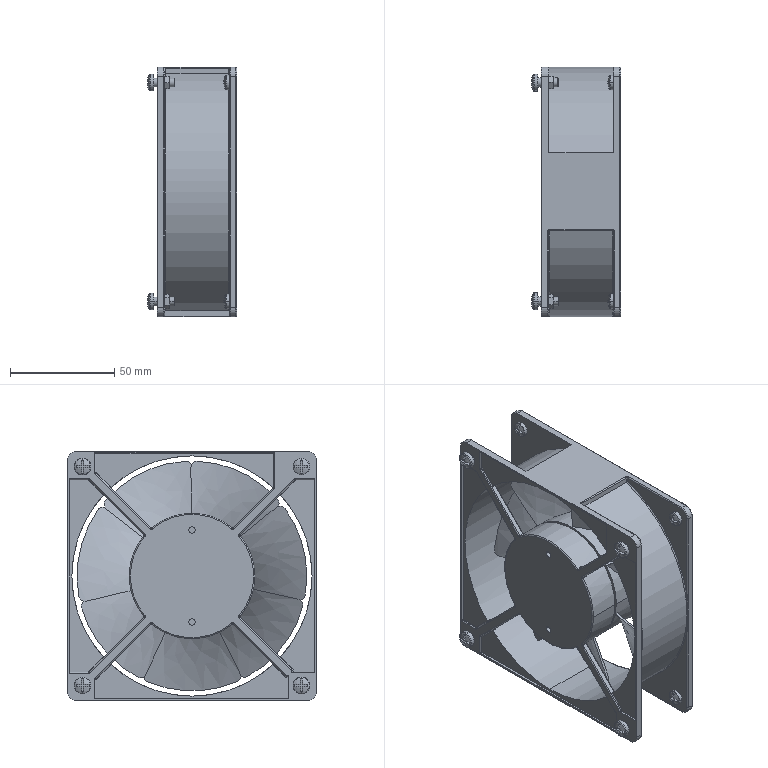Part | STEP file | FKL6622 cabinet fan and filter[FKL6622.230]_120_G8025HA1S | 1 solid | 562 faces | box 42.957 x 119.523 x 119.5 mm | volume 164726 mm3 | plane 216 | cylinder 170 | torus 78 | spline 56 | cone 26 | sphere 16 | commonest cylinder face diameters 1 x94 4.2 x26 8 x10 6 x9 7 x8 8.8 x8